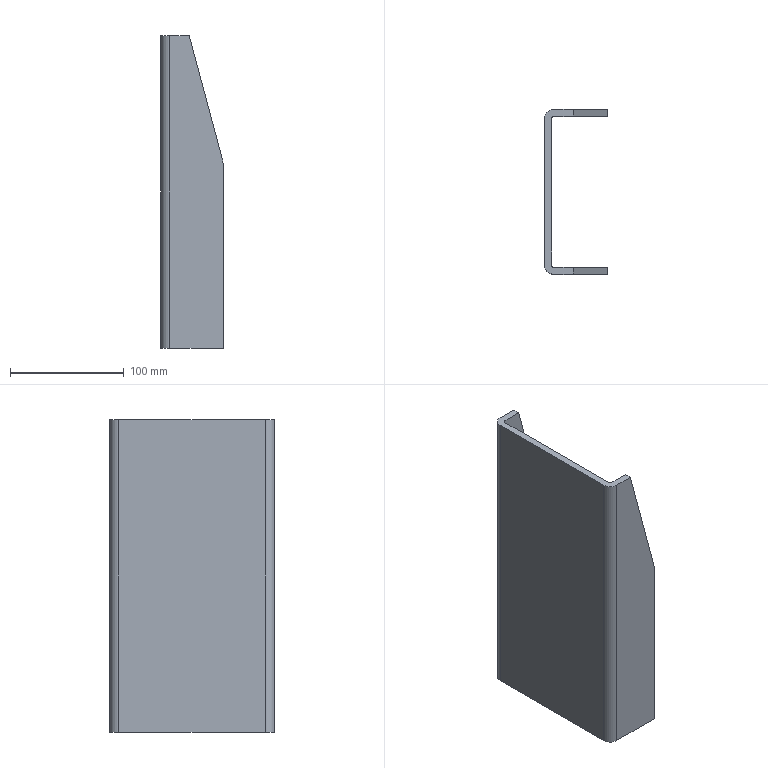Part | SolidWorks | features Extrusion 1, ICE 1 | 1 solid | 16 faces | box 55 x 145 x 275 mm | volume 373708 mm3 | plane 12 | cylinder 4 | commonest cylinder face diameters 4 x2 16 x2
STEP:
#1=CARTESIAN_POINT('',(0.,0.,163.));
#2=VERTEX_POINT('',#1);
#3=CARTESIAN_POINT('',(0.,0.,0.));
#4=VERTEX_POINT('',#3);
#5=CARTESIAN_POINT('',(0.,0.,275.));
#6=DIRECTION('',(0.,0.,-1.));
#7=VECTOR('',#6,1000.);
#8=LINE('',#5,#7);
#9=EDGE_CURVE('',#2,#4,#8,.T.);
#10=ORIENTED_EDGE('',*,*,#9,.F.);
#11=CARTESIAN_POINT('',(0.,-6.,163.));
#12=VERTEX_POINT('',#11);
#13=CARTESIAN_POINT('',(0.,-275.,163.));
#14=DIRECTION('',(0.,1.,0.));
#15=VECTOR('',#14,1000.);
#16=LINE('',#13,#15);
#17=EDGE_CURVE('',#12,#2,#16,.T.);
#18=ORIENTED_EDGE('',*,*,#17,.F.);
#19=CARTESIAN_POINT('',(0.,-6.,0.));
#20=VERTEX_POINT('',#19);
#21=CARTESIAN_POINT('',(0.,-6.,275.));
#22=DIRECTION('',(0.,0.,-1.));
#23=VECTOR('',#22,1000.);
#24=LINE('',#21,#23);
#25=EDGE_CURVE('',#12,#20,#24,.T.);
#26=ORIENTED_EDGE('',*,*,#25,.T.);
#27=CARTESIAN_POINT('',(0.,0.,0.));
#28=DIRECTION('',(0.,1.,0.));
#29=VECTOR('',#28,1000.);
#30=LINE('',#27,#29);
#31=EDGE_CURVE('',#20,#4,#30,.T.);
#32=ORIENTED_EDGE('',*,*,#31,.T.);
#33=EDGE_LOOP('',(#10,#18,#26,#32));
#34=FACE_OUTER_BOUND('',#33,.T.);
#35=CARTESIAN_POINT('',(0.,0.,275.));
#36=DIRECTION('',(-1.,0.,0.));
#37=DIRECTION('',(0.,0.,1.));
#38=AXIS2_PLACEMENT_3D('',#35,#36,#37);
#39=PLANE('',#38);
#40=ADVANCED_FACE('',(#34),#39,.F.);
#41=CARTESIAN_POINT('',(-30.,0.,275.));
#42=VERTEX_POINT('',#41);
#43=CARTESIAN_POINT('',(-47.,0.,275.));
#44=VERTEX_POINT('',#43);
#45=CARTESIAN_POINT('',(0.,0.,275.));
#46=DIRECTION('',(-1.,0.,0.));
#47=VECTOR('',#46,1000.);
#48=LINE('',#45,#47);
#49=EDGE_CURVE('',#42,#44,#48,.T.);
#50=ORIENTED_EDGE('',*,*,#49,.F.);
#51=CARTESIAN_POINT('',(0.,0.,163.));
#52=DIRECTION('',(-0.2587,0.,0.9659));
#53=VECTOR('',#52,1000.);
#54=LINE('',#51,#53);
#55=EDGE_CURVE('',#2,#42,#54,.T.);
#56=ORIENTED_EDGE('',*,*,#55,.F.);
#57=ORIENTED_EDGE('',*,*,#9,.T.);
#58=CARTESIAN_POINT('',(-47.,0.,0.));
#59=VERTEX_POINT('',#58);
#60=CARTESIAN_POINT('',(0.,0.,0.));
#61=DIRECTION('',(-1.,0.,0.));
#62=VECTOR('',#61,1000.);
#63=LINE('',#60,#62);
#64=EDGE_CURVE('',#4,#59,#63,.T.);
#65=ORIENTED_EDGE('',*,*,#64,.T.);
#66=CARTESIAN_POINT('',(-47.,0.,275.));
#67=DIRECTION('',(0.,0.,-1.));
#68=VECTOR('',#67,1000.);
#69=LINE('',#66,#68);
#70=EDGE_CURVE('',#44,#59,#69,.T.);
#71=ORIENTED_EDGE('',*,*,#70,.F.);
#72=EDGE_LOOP('',(#50,#56,#57,#65,#71));
#73=FACE_OUTER_BOUND('',#72,.T.);
#74=CARTESIAN_POINT('',(0.,0.,275.));
#75=DIRECTION('',(0.,-1.,0.));
#76=DIRECTION('',(0.,0.,-1.));
#77=AXIS2_PLACEMENT_3D('',#74,#75,#76);
#78=PLANE('',#77);
#79=ADVANCED_FACE('',(#73),#78,.F.);
#80=CARTESIAN_POINT('',(-55.,-8.,0.));
#81=VERTEX_POINT('',#80);
#82=CARTESIAN_POINT('',(-47.,-8.,0.));
#83=DIRECTION('',(0.,0.,1.));
#84=DIRECTION('',(1.,0.,0.));
#85=AXIS2_PLACEMENT_3D('',#82,#83,#84);
#86=CIRCLE('',#85,8.);
#87=EDGE_CURVE('',#59,#81,#86,.T.);
#88=ORIENTED_EDGE('',*,*,#87,.T.);
#89=CARTESIAN_POINT('',(-55.,-8.,275.));
#90=VERTEX_POINT('',#89);
#91=CARTESIAN_POINT('',(-55.,-8.,275.));
#92=DIRECTION('',(0.,0.,-1.));
#93=VECTOR('',#92,1000.);
#94=LINE('',#91,#93);
#95=EDGE_CURVE('',#90,#81,#94,.T.);
#96=ORIENTED_EDGE('',*,*,#95,.F.);
#97=CARTESIAN_POINT('',(-47.,-8.,275.));
#98=DIRECTION('',(0.,0.,1.));
#99=DIRECTION('',(1.,0.,0.));
#100=AXIS2_PLACEMENT_3D('',#97,#98,#99);
#101=CIRCLE('',#100,8.);
#102=EDGE_CURVE('',#44,#90,#101,.T.);
#103=ORIENTED_EDGE('',*,*,#102,.F.);
#104=ORIENTED_EDGE('',*,*,#70,.T.);
#105=EDGE_LOOP('',(#88,#96,#103,#104));
#106=FACE_OUTER_BOUND('',#105,.T.);
#107=CARTESIAN_POINT('',(-47.,-8.,275.));
#108=DIRECTION('',(0.,0.,-1.));
#109=DIRECTION('',(-1.,0.,0.));
#110=AXIS2_PLACEMENT_3D('',#107,#108,#109);
#111=CYLINDRICAL_SURFACE('',#110,8.);
#112=ADVANCED_FACE('',(#106),#111,.T.);
#113=CARTESIAN_POINT('',(-55.,-137.,0.));
#114=VERTEX_POINT('',#113);
#115=CARTESIAN_POINT('',(-55.,-8.,0.));
#116=DIRECTION('',(0.,-1.,0.));
#117=VECTOR('',#116,1000.);
#118=LINE('',#115,#117);
#119=EDGE_CURVE('',#81,#114,#118,.T.);
#120=ORIENTED_EDGE('',*,*,#119,.T.);
#121=CARTESIAN_POINT('',(-55.,-137.,275.));
#122=VERTEX_POINT('',#121);
#123=CARTESIAN_POINT('',(-55.,-137.,275.));
#124=DIRECTION('',(0.,0.,-1.));
#125=VECTOR('',#124,1000.);
#126=LINE('',#123,#125);
#127=EDGE_CURVE('',#122,#114,#126,.T.);
#128=ORIENTED_EDGE('',*,*,#127,.F.);
#129=CARTESIAN_POINT('',(-55.,-8.,275.));
#130=DIRECTION('',(0.,-1.,0.));
#131=VECTOR('',#130,1000.);
#132=LINE('',#129,#131);
#133=EDGE_CURVE('',#90,#122,#132,.T.);
#134=ORIENTED_EDGE('',*,*,#133,.F.);
#135=ORIENTED_EDGE('',*,*,#95,.T.);
#136=EDGE_LOOP('',(#120,#128,#134,#135));
#137=FACE_OUTER_BOUND('',#136,.T.);
#138=CARTESIAN_POINT('',(-55.,-8.,275.));
#139=DIRECTION('',(1.,0.,0.));
#140=DIRECTION('',(0.,1.,0.));
#141=AXIS2_PLACEMENT_3D('',#138,#139,#140);
#142=PLANE('',#141);
#143=ADVANCED_FACE('',(#137),#142,.F.);
#144=CARTESIAN_POINT('',(-47.,-145.,0.));
#145=VERTEX_POINT('',#144);
#146=CARTESIAN_POINT('',(-47.,-137.,0.));
#147=DIRECTION('',(0.,0.,1.));
#148=DIRECTION('',(1.,0.,0.));
#149=AXIS2_PLACEMENT_3D('',#146,#147,#148);
#150=CIRCLE('',#149,8.);
#151=EDGE_CURVE('',#114,#145,#150,.T.);
#152=ORIENTED_EDGE('',*,*,#151,.T.);
#153=CARTESIAN_POINT('',(-47.,-145.,275.));
#154=VERTEX_POINT('',#153);
#155=CARTESIAN_POINT('',(-47.,-145.,275.));
#156=DIRECTION('',(0.,0.,-1.));
#157=VECTOR('',#156,1000.);
#158=LINE('',#155,#157);
#159=EDGE_CURVE('',#154,#145,#158,.T.);
#160=ORIENTED_EDGE('',*,*,#159,.F.);
#161=CARTESIAN_POINT('',(-47.,-137.,275.));
#162=DIRECTION('',(0.,0.,1.));
#163=DIRECTION('',(1.,0.,0.));
#164=AXIS2_PLACEMENT_3D('',#161,#162,#163);
#165=CIRCLE('',#164,8.);
#166=EDGE_CURVE('',#122,#154,#165,.T.);
#167=ORIENTED_EDGE('',*,*,#166,.F.);
#168=ORIENTED_EDGE('',*,*,#127,.T.);
#169=EDGE_LOOP('',(#152,#160,#167,#168));
#170=FACE_OUTER_BOUND('',#169,.T.);
#171=CARTESIAN_POINT('',(-47.,-137.,275.));
#172=DIRECTION('',(0.,0.,-1.));
#173=DIRECTION('',(-1.,0.,0.));
#174=AXIS2_PLACEMENT_3D('',#171,#172,#173);
#175=CYLINDRICAL_SURFACE('',#174,8.);
#176=ADVANCED_FACE('',(#170),#175,.T.);
#177=CARTESIAN_POINT('',(0.,-145.,163.));
#178=VERTEX_POINT('',#177);
#179=CARTESIAN_POINT('',(0.,-145.,0.));
#180=VERTEX_POINT('',#179);
#181=CARTESIAN_POINT('',(0.,-145.,275.));
#182=DIRECTION('',(0.,0.,-1.));
#183=VECTOR('',#182,1000.);
#184=LINE('',#181,#183);
#185=EDGE_CURVE('',#178,#180,#184,.T.);
#186=ORIENTED_EDGE('',*,*,#185,.F.);
#187=CARTESIAN_POINT('',(-30.,-145.,275.));
#188=VERTEX_POINT('',#187);
#189=CARTESIAN_POINT('',(-31.138,-145.,279.249));
#190=DIRECTION('',(-0.2587,0.,0.9659));
#191=VECTOR('',#190,1000.);
#192=LINE('',#189,#191);
#193=EDGE_CURVE('',#178,#188,#192,.T.);
#194=ORIENTED_EDGE('',*,*,#193,.T.);
#195=CARTESIAN_POINT('',(-47.,-145.,275.));
#196=DIRECTION('',(1.,0.,0.));
#197=VECTOR('',#196,1000.);
#198=LINE('',#195,#197);
#199=EDGE_CURVE('',#154,#188,#198,.T.);
#200=ORIENTED_EDGE('',*,*,#199,.F.);
#201=ORIENTED_EDGE('',*,*,#159,.T.);
#202=CARTESIAN_POINT('',(-47.,-145.,0.));
#203=DIRECTION('',(1.,0.,0.));
#204=VECTOR('',#203,1000.);
#205=LINE('',#202,#204);
#206=EDGE_CURVE('',#145,#180,#205,.T.);
#207=ORIENTED_EDGE('',*,*,#206,.T.);
#208=EDGE_LOOP('',(#186,#194,#200,#201,#207));
#209=FACE_OUTER_BOUND('',#208,.T.);
#210=CARTESIAN_POINT('',(-47.,-145.,275.));
#211=DIRECTION('',(0.,1.,0.));
#212=DIRECTION('',(0.,0.,1.));
#213=AXIS2_PLACEMENT_3D('',#210,#211,#212);
#214=PLANE('',#213);
#215=ADVANCED_FACE('',(#209),#214,.F.);
#216=CARTESIAN_POINT('',(0.,-139.,163.));
#217=VERTEX_POINT('',#216);
#218=CARTESIAN_POINT('',(0.,-139.,0.));
#219=VERTEX_POINT('',#218);
#220=CARTESIAN_POINT('',(0.,-139.,275.));
#221=DIRECTION('',(0.,0.,-1.));
#222=VECTOR('',#221,1000.);
#223=LINE('',#220,#222);
#224=EDGE_CURVE('',#217,#219,#223,.T.);
#225=ORIENTED_EDGE('',*,*,#224,.F.);
#226=CARTESIAN_POINT('',(0.,-275.,163.));
#227=DIRECTION('',(0.,1.,0.));
#228=VECTOR('',#227,1000.);
#229=LINE('',#226,#228);
#230=EDGE_CURVE('',#178,#217,#229,.T.);
#231=ORIENTED_EDGE('',*,*,#230,.F.);
#232=ORIENTED_EDGE('',*,*,#185,.T.);
#233=CARTESIAN_POINT('',(0.,-139.,0.));
#234=DIRECTION('',(0.,1.,0.));
#235=VECTOR('',#234,1000.);
#236=LINE('',#233,#235);
#237=EDGE_CURVE('',#180,#219,#236,.T.);
#238=ORIENTED_EDGE('',*,*,#237,.T.);
#239=EDGE_LOOP('',(#225,#231,#232,#238));
#240=FACE_OUTER_BOUND('',#239,.T.);
#241=CARTESIAN_POINT('',(0.,-139.,275.));
#242=DIRECTION('',(-1.,0.,0.));
#243=DIRECTION('',(0.,0.,1.));
#244=AXIS2_PLACEMENT_3D('',#241,#242,#243);
#245=PLANE('',#244);
#246=ADVANCED_FACE('',(#240),#245,.F.);
#247=CARTESIAN_POINT('',(-30.,-139.,275.));
#248=VERTEX_POINT('',#247);
#249=CARTESIAN_POINT('',(-47.,-139.,275.));
#250=VERTEX_POINT('',#249);
#251=CARTESIAN_POINT('',(-47.,-139.,275.));
#252=DIRECTION('',(-1.,0.,0.));
#253=VECTOR('',#252,1000.);
#254=LINE('',#251,#253);
#255=EDGE_CURVE('',#248,#250,#254,.T.);
#256=ORIENTED_EDGE('',*,*,#255,.F.);
#257=CARTESIAN_POINT('',(-31.138,-139.,279.249));
#258=DIRECTION('',(0.2587,0.,-0.9659));
#259=VECTOR('',#258,1000.);
#260=LINE('',#257,#259);
#261=EDGE_CURVE('',#248,#217,#260,.T.);
#262=ORIENTED_EDGE('',*,*,#261,.T.);
#263=ORIENTED_EDGE('',*,*,#224,.T.);
#264=CARTESIAN_POINT('',(-47.,-139.,0.));
#265=VERTEX_POINT('',#264);
#266=CARTESIAN_POINT('',(-47.,-139.,0.));
#267=DIRECTION('',(-1.,0.,0.));
#268=VECTOR('',#267,1000.);
#269=LINE('',#266,#268);
#270=EDGE_CURVE('',#219,#265,#269,.T.);
#271=ORIENTED_EDGE('',*,*,#270,.T.);
#272=CARTESIAN_POINT('',(-47.,-139.,275.));
#273=DIRECTION('',(0.,0.,-1.));
#274=VECTOR('',#273,1000.);
#275=LINE('',#272,#274);
#276=EDGE_CURVE('',#250,#265,#275,.T.);
#277=ORIENTED_EDGE('',*,*,#276,.F.);
#278=EDGE_LOOP('',(#256,#262,#263,#271,#277));
#279=FACE_OUTER_BOUND('',#278,.T.);
#280=CARTESIAN_POINT('',(-47.,-139.,275.));
#281=DIRECTION('',(0.,-1.,0.));
#282=DIRECTION('',(0.,0.,-1.));
#283=AXIS2_PLACEMENT_3D('',#280,#281,#282);
#284=PLANE('',#283);
#285=ADVANCED_FACE('',(#279),#284,.F.);
#286=CARTESIAN_POINT('',(-49.,-137.,0.));
#287=VERTEX_POINT('',#286);
#288=CARTESIAN_POINT('',(-47.,-137.,0.));
#289=DIRECTION('',(0.,0.,-1.));
#290=DIRECTION('',(1.,0.,0.));
#291=AXIS2_PLACEMENT_3D('',#288,#289,#290);
#292=CIRCLE('',#291,2.);
#293=EDGE_CURVE('',#265,#287,#292,.T.);
#294=ORIENTED_EDGE('',*,*,#293,.T.);
#295=CARTESIAN_POINT('',(-49.,-137.,275.));
#296=VERTEX_POINT('',#295);
#297=CARTESIAN_POINT('',(-49.,-137.,275.));
#298=DIRECTION('',(0.,0.,-1.));
#299=VECTOR('',#298,1000.);
#300=LINE('',#297,#299);
#301=EDGE_CURVE('',#296,#287,#300,.T.);
#302=ORIENTED_EDGE('',*,*,#301,.F.);
#303=CARTESIAN_POINT('',(-47.,-137.,275.));
#304=DIRECTION('',(0.,0.,-1.));
#305=DIRECTION('',(1.,0.,0.));
#306=AXIS2_PLACEMENT_3D('',#303,#304,#305);
#307=CIRCLE('',#306,2.);
#308=EDGE_CURVE('',#250,#296,#307,.T.);
#309=ORIENTED_EDGE('',*,*,#308,.F.);
#310=ORIENTED_EDGE('',*,*,#276,.T.);
#311=EDGE_LOOP('',(#294,#302,#309,#310));
#312=FACE_OUTER_BOUND('',#311,.T.);
#313=CARTESIAN_POINT('',(-47.,-137.,275.));
#314=DIRECTION('',(0.,0.,-1.));
#315=DIRECTION('',(-1.,0.,0.));
#316=AXIS2_PLACEMENT_3D('',#313,#314,#315);
#317=CYLINDRICAL_SURFACE('',#316,2.);
#318=ADVANCED_FACE('',(#312),#317,.F.);
#319=CARTESIAN_POINT('',(-49.,-8.,0.));
#320=VERTEX_POINT('',#319);
#321=CARTESIAN_POINT('',(-49.,-8.,0.));
#322=DIRECTION('',(0.,1.,0.));
#323=VECTOR('',#322,1000.);
#324=LINE('',#321,#323);
#325=EDGE_CURVE('',#287,#320,#324,.T.);
#326=ORIENTED_EDGE('',*,*,#325,.T.);
#327=CARTESIAN_POINT('',(-49.,-8.,275.));
#328=VERTEX_POINT('',#327);
#329=CARTESIAN_POINT('',(-49.,-8.,275.));
#330=DIRECTION('',(0.,0.,-1.));
#331=VECTOR('',#330,1000.);
#332=LINE('',#329,#331);
#333=EDGE_CURVE('',#328,#320,#332,.T.);
#334=ORIENTED_EDGE('',*,*,#333,.F.);
#335=CARTESIAN_POINT('',(-49.,-8.,275.));
#336=DIRECTION('',(0.,1.,0.));
#337=VECTOR('',#336,1000.);
#338=LINE('',#335,#337);
#339=EDGE_CURVE('',#296,#328,#338,.T.);
#340=ORIENTED_EDGE('',*,*,#339,.F.);
#341=ORIENTED_EDGE('',*,*,#301,.T.);
#342=EDGE_LOOP('',(#326,#334,#340,#341));
#343=FACE_OUTER_BOUND('',#342,.T.);
#344=CARTESIAN_POINT('',(-49.,-8.,275.));
#345=DIRECTION('',(-1.,0.,0.));
#346=DIRECTION('',(0.,0.,1.));
#347=AXIS2_PLACEMENT_3D('',#344,#345,#346);
#348=PLANE('',#347);
#349=ADVANCED_FACE('',(#343),#348,.F.);
#350=CARTESIAN_POINT('',(-47.,-6.,0.));
#351=VERTEX_POINT('',#350);
#352=CARTESIAN_POINT('',(-47.,-8.,0.));
#353=DIRECTION('',(0.,0.,-1.));
#354=DIRECTION('',(1.,0.,0.));
#355=AXIS2_PLACEMENT_3D('',#352,#353,#354);
#356=CIRCLE('',#355,2.);
#357=EDGE_CURVE('',#320,#351,#356,.T.);
#358=ORIENTED_EDGE('',*,*,#357,.T.);
#359=CARTESIAN_POINT('',(-47.,-6.,275.));
#360=VERTEX_POINT('',#359);
#361=CARTESIAN_POINT('',(-47.,-6.,275.));
#362=DIRECTION('',(0.,0.,-1.));
#363=VECTOR('',#362,1000.);
#364=LINE('',#361,#363);
#365=EDGE_CURVE('',#360,#351,#364,.T.);
#366=ORIENTED_EDGE('',*,*,#365,.F.);
#367=CARTESIAN_POINT('',(-47.,-8.,275.));
#368=DIRECTION('',(0.,0.,-1.));
#369=DIRECTION('',(1.,0.,0.));
#370=AXIS2_PLACEMENT_3D('',#367,#368,#369);
#371=CIRCLE('',#370,2.);
#372=EDGE_CURVE('',#328,#360,#371,.T.);
#373=ORIENTED_EDGE('',*,*,#372,.F.);
#374=ORIENTED_EDGE('',*,*,#333,.T.);
#375=EDGE_LOOP('',(#358,#366,#373,#374));
#376=FACE_OUTER_BOUND('',#375,.T.);
#377=CARTESIAN_POINT('',(-47.,-8.,275.));
#378=DIRECTION('',(0.,0.,-1.));
#379=DIRECTION('',(-1.,0.,0.));
#380=AXIS2_PLACEMENT_3D('',#377,#378,#379);
#381=CYLINDRICAL_SURFACE('',#380,2.);
#382=ADVANCED_FACE('',(#376),#381,.F.);
#383=ORIENTED_EDGE('',*,*,#25,.F.);
#384=CARTESIAN_POINT('',(-30.,-6.,275.));
#385=VERTEX_POINT('',#384);
#386=CARTESIAN_POINT('',(-27.992,-6.,267.502));
#387=DIRECTION('',(-0.2587,0.,0.9659));
#388=VECTOR('',#387,1000.);
#389=LINE('',#386,#388);
#390=EDGE_CURVE('',#12,#385,#389,.T.);
#391=ORIENTED_EDGE('',*,*,#390,.T.);
#392=CARTESIAN_POINT('',(0.,-6.,275.));
#393=DIRECTION('',(1.,0.,0.));
#394=VECTOR('',#393,1000.);
#395=LINE('',#392,#394);
#396=EDGE_CURVE('',#360,#385,#395,.T.);
#397=ORIENTED_EDGE('',*,*,#396,.F.);
#398=ORIENTED_EDGE('',*,*,#365,.T.);
#399=CARTESIAN_POINT('',(0.,-6.,0.));
#400=DIRECTION('',(1.,0.,0.));
#401=VECTOR('',#400,1000.);
#402=LINE('',#399,#401);
#403=EDGE_CURVE('',#351,#20,#402,.T.);
#404=ORIENTED_EDGE('',*,*,#403,.T.);
#405=EDGE_LOOP('',(#383,#391,#397,#398,#404));
#406=FACE_OUTER_BOUND('',#405,.T.);
#407=CARTESIAN_POINT('',(0.,-6.,275.));
#408=DIRECTION('',(0.,1.,0.));
#409=DIRECTION('',(0.,0.,1.));
#410=AXIS2_PLACEMENT_3D('',#407,#408,#409);
#411=PLANE('',#410);
#412=ADVANCED_FACE('',(#406),#411,.F.);
#413=CARTESIAN_POINT('',(-30.,-8.,275.));
#414=DIRECTION('',(0.,-1.,0.));
#415=VECTOR('',#414,1000.);
#416=LINE('',#413,#415);
#417=EDGE_CURVE('',#42,#385,#416,.T.);
#418=ORIENTED_EDGE('',*,*,#417,.F.);
#419=ORIENTED_EDGE('',*,*,#49,.T.);
#420=ORIENTED_EDGE('',*,*,#102,.T.);
#421=ORIENTED_EDGE('',*,*,#133,.T.);
#422=ORIENTED_EDGE('',*,*,#166,.T.);
#423=ORIENTED_EDGE('',*,*,#199,.T.);
#424=CARTESIAN_POINT('',(-30.,-8.,275.));
#425=DIRECTION('',(0.,-1.,0.));
#426=VECTOR('',#425,1000.);
#427=LINE('',#424,#426);
#428=EDGE_CURVE('',#248,#188,#427,.T.);
#429=ORIENTED_EDGE('',*,*,#428,.F.);
#430=ORIENTED_EDGE('',*,*,#255,.T.);
#431=ORIENTED_EDGE('',*,*,#308,.T.);
#432=ORIENTED_EDGE('',*,*,#339,.T.);
#433=ORIENTED_EDGE('',*,*,#372,.T.);
#434=ORIENTED_EDGE('',*,*,#396,.T.);
#435=EDGE_LOOP('',(#418,#419,#420,#421,#422,#423,#429,#430,#431,#432,#433,#434));
#436=FACE_OUTER_BOUND('',#435,.T.);
#437=CARTESIAN_POINT('',(-47.,-8.,275.));
#438=DIRECTION('',(0.,0.,1.));
#439=DIRECTION('',(1.,0.,0.));
#440=AXIS2_PLACEMENT_3D('',#437,#438,#439);
#441=PLANE('',#440);
#442=ADVANCED_FACE('',(#436),#441,.T.);
#443=ORIENTED_EDGE('',*,*,#31,.F.);
#444=ORIENTED_EDGE('',*,*,#403,.F.);
#445=ORIENTED_EDGE('',*,*,#357,.F.);
#446=ORIENTED_EDGE('',*,*,#325,.F.);
#447=ORIENTED_EDGE('',*,*,#293,.F.);
#448=ORIENTED_EDGE('',*,*,#270,.F.);
#449=ORIENTED_EDGE('',*,*,#237,.F.);
#450=ORIENTED_EDGE('',*,*,#206,.F.);
#451=ORIENTED_EDGE('',*,*,#151,.F.);
#452=ORIENTED_EDGE('',*,*,#119,.F.);
#453=ORIENTED_EDGE('',*,*,#87,.F.);
#454=ORIENTED_EDGE('',*,*,#64,.F.);
#455=EDGE_LOOP('',(#443,#444,#445,#446,#447,#448,#449,#450,#451,#452,#453,#454));
#456=FACE_OUTER_BOUND('',#455,.T.);
#457=CARTESIAN_POINT('',(-47.,-8.,0.));
#458=DIRECTION('',(0.,0.,1.));
#459=DIRECTION('',(1.,0.,0.));
#460=AXIS2_PLACEMENT_3D('',#457,#458,#459);
#461=PLANE('',#460);
#462=ADVANCED_FACE('',(#456),#461,.F.);
#463=ORIENTED_EDGE('',*,*,#230,.T.);
#464=ORIENTED_EDGE('',*,*,#261,.F.);
#465=ORIENTED_EDGE('',*,*,#428,.T.);
#466=ORIENTED_EDGE('',*,*,#193,.F.);
#467=EDGE_LOOP('',(#463,#464,#465,#466));
#468=FACE_OUTER_BOUND('',#467,.T.);
#469=CARTESIAN_POINT('',(0.,-275.,163.));
#470=DIRECTION('',(-0.9659,0.,-0.2587));
#471=DIRECTION('',(-0.2587,0.,0.9659));
#472=AXIS2_PLACEMENT_3D('',#469,#470,#471);
#473=PLANE('',#472);
#474=ADVANCED_FACE('',(#468),#473,.F.);
#475=ORIENTED_EDGE('',*,*,#17,.T.);
#476=ORIENTED_EDGE('',*,*,#55,.T.);
#477=ORIENTED_EDGE('',*,*,#417,.T.);
#478=ORIENTED_EDGE('',*,*,#390,.F.);
#479=EDGE_LOOP('',(#475,#476,#477,#478));
#480=FACE_OUTER_BOUND('',#479,.T.);
#481=CARTESIAN_POINT('',(0.,-275.,163.));
#482=DIRECTION('',(-0.9659,0.,-0.2587));
#483=DIRECTION('',(-0.2587,0.,0.9659));
#484=AXIS2_PLACEMENT_3D('',#481,#482,#483);
#485=PLANE('',#484);
#486=ADVANCED_FACE('',(#480),#485,.F.);
#487=CLOSED_SHELL('',(#40,#79,#112,#143,#176,#215,#246,#285,#318,#349,#382,#412,#442,#462,#474,#486));
#488=MANIFOLD_SOLID_BREP('',#487);
#489=CARTESIAN_POINT('',(0.,0.,0.));
#490=DIRECTION('',(0.,0.,1.));
#491=DIRECTION('',(1.,0.,0.));
#492=AXIS2_PLACEMENT_3D('',#489,#490,#491);
#493=(LENGTH_UNIT()NAMED_UNIT(*)SI_UNIT(.MILLI.,.METRE.));
#494=UNCERTAINTY_MEASURE_WITH_UNIT(LENGTH_MEASURE(0.00001),#493,'','');
#495=(NAMED_UNIT(*)PLANE_ANGLE_UNIT()SI_UNIT($,.RADIAN.));
#496=(NAMED_UNIT(*)SI_UNIT($,.STERADIAN.)SOLID_ANGLE_UNIT());
#497=(GEOMETRIC_REPRESENTATION_CONTEXT(3)GLOBAL_UNCERTAINTY_ASSIGNED_CONTEXT((#494))GLOBAL_UNIT_ASSIGNED_CONTEXT((#493,#495,#496))REPRESENTATION_CONTEXT('',''));
#498=ADVANCED_BREP_SHAPE_REPRESENTATION('',(#488,#492),#497);